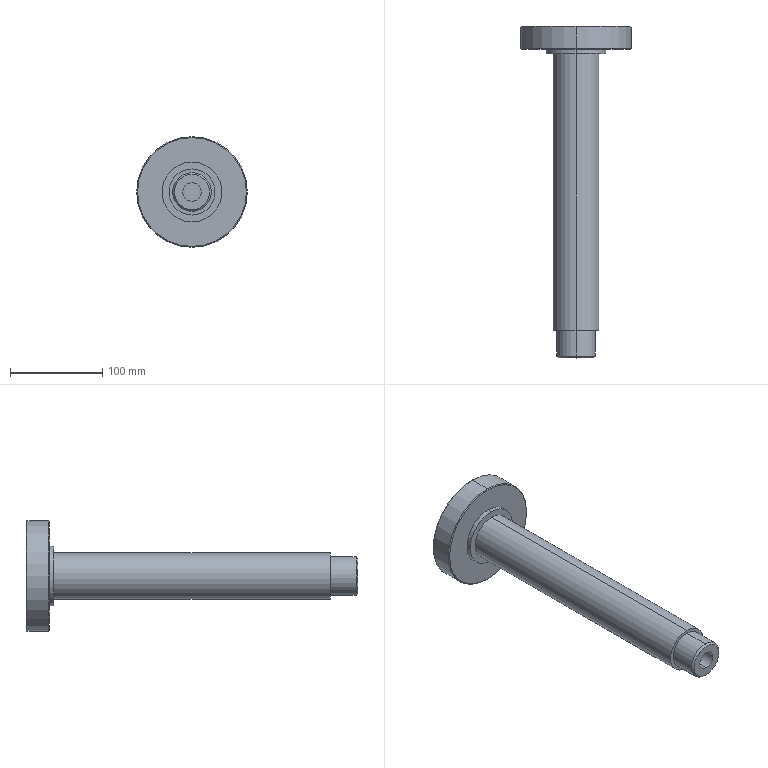Part | STEP file | Backup 2012-3-22-04 | 1 solid | 22 faces | box 120 x 360 x 120 mm | volume 913608 mm3 | cylinder 10 | cone 6 | plane 6 | commonest cylinder face diameters 20 x2 42 x2 50 x2 65 x2 120 x2
STEP:
#1=CARTESIAN_POINT('',(0.,0.,0.));
#2=DIRECTION('',(0.,0.,1.));
#3=DIRECTION('',(1.,0.,0.));
#4=AXIS2_PLACEMENT_3D('',#1,#2,#3);
#5=CARTESIAN_POINT('',(0.,0.,-19.));
#6=VERTEX_POINT('',#5);
#7=CARTESIAN_POINT('',(0.,0.,19.));
#8=VERTEX_POINT('',#7);
#9=CARTESIAN_POINT('',(0.,0.,0.));
#10=DIRECTION('',(0.,-1.,0.));
#11=DIRECTION('',(0.,0.,-1.));
#12=AXIS2_PLACEMENT_3D('',#9,#10,#11);
#13=CIRCLE('',#12,19.);
#14=CARTESIAN_POINT('',(0.,0.,0.));
#15=DIRECTION('',(0.,1.,0.));
#16=DIRECTION('',(0.,0.,1.));
#17=AXIS2_PLACEMENT_3D('',#14,#15,#16);
#18=CONICAL_SURFACE('',#17,19.,0.7854);
#19=CARTESIAN_POINT('',(3.142,0.));
#20=DIRECTION('',(-1.,0.));
#21=VECTOR('',#20,1.);
#22=LINE('',#19,#21);
#23=(GEOMETRIC_REPRESENTATION_CONTEXT(2)PARAMETRIC_REPRESENTATION_CONTEXT()REPRESENTATION_CONTEXT('',''));
#24=DEFINITIONAL_REPRESENTATION('',(#22),#23);
#25=PCURVE('',#18,#24);
#26=CARTESIAN_POINT('',(10.,0.,0.));
#27=DIRECTION('',(0.,-1.,0.));
#28=DIRECTION('',(0.,0.,-1.));
#29=AXIS2_PLACEMENT_3D('',#26,#27,#28);
#30=PLANE('',#29);
#31=CARTESIAN_POINT('',(0.,-10.));
#32=DIRECTION('',(1.,0.));
#33=AXIS2_PLACEMENT_2D('',#31,#32);
#34=CIRCLE('',#33,19.);
#35=(GEOMETRIC_REPRESENTATION_CONTEXT(2)PARAMETRIC_REPRESENTATION_CONTEXT()REPRESENTATION_CONTEXT('',''));
#36=DEFINITIONAL_REPRESENTATION('',(#34),#35);
#37=PCURVE('',#30,#36);
#38=SURFACE_CURVE('',#13,(#25,#37),.PCURVE_S1.);
#39=EDGE_CURVE('',#6,#8,#38,.T.);
#40=ORIENTED_EDGE('',*,*,#39,.F.);
#41=CARTESIAN_POINT('',(0.,2.,-21.));
#42=VERTEX_POINT('',#41);
#43=CARTESIAN_POINT('',(0.,0.,-19.));
#44=DIRECTION('',(0.,0.7071,-0.7071));
#45=VECTOR('',#44,1.);
#46=LINE('',#43,#45);
#47=CARTESIAN_POINT('',(3.142,0.));
#48=DIRECTION('',(0.,1.));
#49=VECTOR('',#48,1.);
#50=LINE('',#47,#49);
#51=(GEOMETRIC_REPRESENTATION_CONTEXT(2)PARAMETRIC_REPRESENTATION_CONTEXT()REPRESENTATION_CONTEXT('',''));
#52=DEFINITIONAL_REPRESENTATION('',(#50),#51);
#53=PCURVE('',#18,#52);
#54=CARTESIAN_POINT('',(0.,0.,0.));
#55=DIRECTION('',(0.,1.,0.));
#56=DIRECTION('',(0.,0.,1.));
#57=AXIS2_PLACEMENT_3D('',#54,#55,#56);
#58=CONICAL_SURFACE('',#57,19.,0.7854);
#59=CARTESIAN_POINT('',(3.142,0.));
#60=DIRECTION('',(0.,1.));
#61=VECTOR('',#60,1.);
#62=LINE('',#59,#61);
#63=(GEOMETRIC_REPRESENTATION_CONTEXT(2)PARAMETRIC_REPRESENTATION_CONTEXT()REPRESENTATION_CONTEXT('',''));
#64=DEFINITIONAL_REPRESENTATION('',(#62),#63);
#65=PCURVE('',#58,#64);
#66=SURFACE_CURVE('',#46,(#53,#65),.PCURVE_S1.);
#67=EDGE_CURVE('',#6,#42,#66,.T.);
#68=ORIENTED_EDGE('',*,*,#67,.T.);
#69=CARTESIAN_POINT('',(0.,2.,21.));
#70=VERTEX_POINT('',#69);
#71=CARTESIAN_POINT('',(0.,2.,0.));
#72=DIRECTION('',(0.,1.,0.));
#73=DIRECTION('',(0.,0.,-1.));
#74=AXIS2_PLACEMENT_3D('',#71,#72,#73);
#75=CIRCLE('',#74,21.);
#76=CARTESIAN_POINT('',(-3.142,2.));
#77=DIRECTION('',(1.,0.));
#78=VECTOR('',#77,1.);
#79=LINE('',#76,#78);
#80=(GEOMETRIC_REPRESENTATION_CONTEXT(2)PARAMETRIC_REPRESENTATION_CONTEXT()REPRESENTATION_CONTEXT('',''));
#81=DEFINITIONAL_REPRESENTATION('',(#79),#80);
#82=PCURVE('',#18,#81);
#83=CARTESIAN_POINT('',(0.,0.,0.));
#84=DIRECTION('',(0.,-1.,0.));
#85=DIRECTION('',(0.,0.,-1.));
#86=AXIS2_PLACEMENT_3D('',#83,#84,#85);
#87=CYLINDRICAL_SURFACE('',#86,21.);
#88=CARTESIAN_POINT('',(6.283,-2.));
#89=DIRECTION('',(-1.,0.));
#90=VECTOR('',#89,1.);
#91=LINE('',#88,#90);
#92=(GEOMETRIC_REPRESENTATION_CONTEXT(2)PARAMETRIC_REPRESENTATION_CONTEXT()REPRESENTATION_CONTEXT('',''));
#93=DEFINITIONAL_REPRESENTATION('',(#91),#92);
#94=PCURVE('',#87,#93);
#95=SURFACE_CURVE('',#75,(#82,#94),.PCURVE_S1.);
#96=EDGE_CURVE('',#70,#42,#95,.T.);
#97=ORIENTED_EDGE('',*,*,#96,.F.);
#98=CARTESIAN_POINT('',(0.,0.,19.));
#99=DIRECTION('',(0.,0.7071,0.7071));
#100=VECTOR('',#99,1.);
#101=LINE('',#98,#100);
#102=CARTESIAN_POINT('',(0.,0.));
#103=DIRECTION('',(0.,1.));
#104=VECTOR('',#103,1.);
#105=LINE('',#102,#104);
#106=(GEOMETRIC_REPRESENTATION_CONTEXT(2)PARAMETRIC_REPRESENTATION_CONTEXT()REPRESENTATION_CONTEXT('',''));
#107=DEFINITIONAL_REPRESENTATION('',(#105),#106);
#108=PCURVE('',#18,#107);
#109=CARTESIAN_POINT('',(6.283,0.));
#110=DIRECTION('',(0.,1.));
#111=VECTOR('',#110,1.);
#112=LINE('',#109,#111);
#113=(GEOMETRIC_REPRESENTATION_CONTEXT(2)PARAMETRIC_REPRESENTATION_CONTEXT()REPRESENTATION_CONTEXT('',''));
#114=DEFINITIONAL_REPRESENTATION('',(#112),#113);
#115=PCURVE('',#58,#114);
#116=SURFACE_CURVE('',#101,(#108,#115),.PCURVE_S1.);
#117=EDGE_CURVE('',#8,#70,#116,.T.);
#118=ORIENTED_EDGE('',*,*,#117,.F.);
#119=EDGE_LOOP('',(#40,#68,#97,#118));
#120=FACE_BOUND('',#119,.T.);
#121=ADVANCED_FACE('',(#120),#18,.T.);
#122=CARTESIAN_POINT('',(0.,360.,59.));
#123=VERTEX_POINT('',#122);
#124=CARTESIAN_POINT('',(0.,360.,-59.));
#125=VERTEX_POINT('',#124);
#126=CARTESIAN_POINT('',(0.,360.,0.));
#127=DIRECTION('',(0.,1.,0.));
#128=DIRECTION('',(0.,0.,1.));
#129=AXIS2_PLACEMENT_3D('',#126,#127,#128);
#130=CIRCLE('',#129,59.);
#131=CARTESIAN_POINT('',(0.,359.,0.));
#132=DIRECTION('',(0.,-1.,0.));
#133=DIRECTION('',(0.,0.,-1.));
#134=AXIS2_PLACEMENT_3D('',#131,#132,#133);
#135=CONICAL_SURFACE('',#134,60.,0.7854);
#136=CARTESIAN_POINT('',(3.142,-1.));
#137=DIRECTION('',(-1.,0.));
#138=VECTOR('',#137,1.);
#139=LINE('',#136,#138);
#140=(GEOMETRIC_REPRESENTATION_CONTEXT(2)PARAMETRIC_REPRESENTATION_CONTEXT()REPRESENTATION_CONTEXT('',''));
#141=DEFINITIONAL_REPRESENTATION('',(#139),#140);
#142=PCURVE('',#135,#141);
#143=CARTESIAN_POINT('',(0.,360.,0.));
#144=DIRECTION('',(0.,1.,0.));
#145=DIRECTION('',(0.,0.,1.));
#146=AXIS2_PLACEMENT_3D('',#143,#144,#145);
#147=PLANE('',#146);
#148=CARTESIAN_POINT('',(0.,0.));
#149=DIRECTION('',(1.,0.));
#150=AXIS2_PLACEMENT_2D('',#148,#149);
#151=CIRCLE('',#150,59.);
#152=(GEOMETRIC_REPRESENTATION_CONTEXT(2)PARAMETRIC_REPRESENTATION_CONTEXT()REPRESENTATION_CONTEXT('',''));
#153=DEFINITIONAL_REPRESENTATION('',(#151),#152);
#154=PCURVE('',#147,#153);
#155=SURFACE_CURVE('',#130,(#142,#154),.PCURVE_S1.);
#156=EDGE_CURVE('',#123,#125,#155,.T.);
#157=ORIENTED_EDGE('',*,*,#156,.F.);
#158=CARTESIAN_POINT('',(0.,359.,60.));
#159=VERTEX_POINT('',#158);
#160=CARTESIAN_POINT('',(0.,359.,60.));
#161=DIRECTION('',(0.,-0.7071,0.7071));
#162=VECTOR('',#161,1.);
#163=LINE('',#160,#162);
#164=CARTESIAN_POINT('',(3.142,0.));
#165=DIRECTION('',(0.,1.));
#166=VECTOR('',#165,1.);
#167=LINE('',#164,#166);
#168=(GEOMETRIC_REPRESENTATION_CONTEXT(2)PARAMETRIC_REPRESENTATION_CONTEXT()REPRESENTATION_CONTEXT('',''));
#169=DEFINITIONAL_REPRESENTATION('',(#167),#168);
#170=PCURVE('',#135,#169);
#171=CARTESIAN_POINT('',(0.,359.,0.));
#172=DIRECTION('',(0.,-1.,0.));
#173=DIRECTION('',(0.,0.,-1.));
#174=AXIS2_PLACEMENT_3D('',#171,#172,#173);
#175=CONICAL_SURFACE('',#174,60.,0.7854);
#176=CARTESIAN_POINT('',(3.142,0.));
#177=DIRECTION('',(0.,1.));
#178=VECTOR('',#177,1.);
#179=LINE('',#176,#178);
#180=(GEOMETRIC_REPRESENTATION_CONTEXT(2)PARAMETRIC_REPRESENTATION_CONTEXT()REPRESENTATION_CONTEXT('',''));
#181=DEFINITIONAL_REPRESENTATION('',(#179),#180);
#182=PCURVE('',#175,#181);
#183=SURFACE_CURVE('',#163,(#170,#182),.PCURVE_S1.);
#184=EDGE_CURVE('',#123,#159,#183,.T.);
#185=ORIENTED_EDGE('',*,*,#184,.T.);
#186=CARTESIAN_POINT('',(0.,359.,-60.));
#187=VERTEX_POINT('',#186);
#188=CARTESIAN_POINT('',(0.,359.,0.));
#189=DIRECTION('',(0.,-1.,0.));
#190=DIRECTION('',(0.,0.,1.));
#191=AXIS2_PLACEMENT_3D('',#188,#189,#190);
#192=CIRCLE('',#191,60.);
#193=CARTESIAN_POINT('',(-3.142,0.));
#194=DIRECTION('',(1.,0.));
#195=VECTOR('',#194,1.);
#196=LINE('',#193,#195);
#197=(GEOMETRIC_REPRESENTATION_CONTEXT(2)PARAMETRIC_REPRESENTATION_CONTEXT()REPRESENTATION_CONTEXT('',''));
#198=DEFINITIONAL_REPRESENTATION('',(#196),#197);
#199=PCURVE('',#135,#198);
#200=CARTESIAN_POINT('',(0.,0.,0.));
#201=DIRECTION('',(0.,-1.,0.));
#202=DIRECTION('',(0.,0.,-1.));
#203=AXIS2_PLACEMENT_3D('',#200,#201,#202);
#204=CYLINDRICAL_SURFACE('',#203,60.);
#205=CARTESIAN_POINT('',(-3.142,-359.));
#206=DIRECTION('',(1.,0.));
#207=VECTOR('',#206,1.);
#208=LINE('',#205,#207);
#209=(GEOMETRIC_REPRESENTATION_CONTEXT(2)PARAMETRIC_REPRESENTATION_CONTEXT()REPRESENTATION_CONTEXT('',''));
#210=DEFINITIONAL_REPRESENTATION('',(#208),#209);
#211=PCURVE('',#204,#210);
#212=SURFACE_CURVE('',#192,(#199,#211),.PCURVE_S1.);
#213=EDGE_CURVE('',#187,#159,#212,.T.);
#214=ORIENTED_EDGE('',*,*,#213,.F.);
#215=CARTESIAN_POINT('',(0.,359.,-60.));
#216=DIRECTION('',(0.,-0.7071,-0.7071));
#217=VECTOR('',#216,1.);
#218=LINE('',#215,#217);
#219=CARTESIAN_POINT('',(0.,0.));
#220=DIRECTION('',(0.,1.));
#221=VECTOR('',#220,1.);
#222=LINE('',#219,#221);
#223=(GEOMETRIC_REPRESENTATION_CONTEXT(2)PARAMETRIC_REPRESENTATION_CONTEXT()REPRESENTATION_CONTEXT('',''));
#224=DEFINITIONAL_REPRESENTATION('',(#222),#223);
#225=PCURVE('',#135,#224);
#226=CARTESIAN_POINT('',(6.283,0.));
#227=DIRECTION('',(0.,1.));
#228=VECTOR('',#227,1.);
#229=LINE('',#226,#228);
#230=(GEOMETRIC_REPRESENTATION_CONTEXT(2)PARAMETRIC_REPRESENTATION_CONTEXT()REPRESENTATION_CONTEXT('',''));
#231=DEFINITIONAL_REPRESENTATION('',(#229),#230);
#232=PCURVE('',#175,#231);
#233=SURFACE_CURVE('',#218,(#225,#232),.PCURVE_S1.);
#234=EDGE_CURVE('',#125,#187,#233,.T.);
#235=ORIENTED_EDGE('',*,*,#234,.F.);
#236=EDGE_LOOP('',(#157,#185,#214,#235));
#237=FACE_BOUND('',#236,.T.);
#238=ADVANCED_FACE('',(#237),#135,.T.);
#239=CARTESIAN_POINT('',(0.,335.,-59.));
#240=VERTEX_POINT('',#239);
#241=CARTESIAN_POINT('',(0.,335.,59.));
#242=VERTEX_POINT('',#241);
#243=CARTESIAN_POINT('',(0.,335.,0.));
#244=DIRECTION('',(0.,-1.,0.));
#245=DIRECTION('',(0.,0.,-1.));
#246=AXIS2_PLACEMENT_3D('',#243,#244,#245);
#247=CIRCLE('',#246,59.);
#248=CARTESIAN_POINT('',(0.,335.,0.));
#249=DIRECTION('',(0.,1.,0.));
#250=DIRECTION('',(0.,0.,1.));
#251=AXIS2_PLACEMENT_3D('',#248,#249,#250);
#252=CONICAL_SURFACE('',#251,59.,0.7854);
#253=CARTESIAN_POINT('',(3.142,0.));
#254=DIRECTION('',(-1.,0.));
#255=VECTOR('',#254,1.);
#256=LINE('',#253,#255);
#257=(GEOMETRIC_REPRESENTATION_CONTEXT(2)PARAMETRIC_REPRESENTATION_CONTEXT()REPRESENTATION_CONTEXT('',''));
#258=DEFINITIONAL_REPRESENTATION('',(#256),#257);
#259=PCURVE('',#252,#258);
#260=CARTESIAN_POINT('',(32.5,335.,0.));
#261=DIRECTION('',(0.,-1.,0.));
#262=DIRECTION('',(0.,0.,-1.));
#263=AXIS2_PLACEMENT_3D('',#260,#261,#262);
#264=PLANE('',#263);
#265=CARTESIAN_POINT('',(0.,-32.5));
#266=DIRECTION('',(1.,0.));
#267=AXIS2_PLACEMENT_2D('',#265,#266);
#268=CIRCLE('',#267,59.);
#269=(GEOMETRIC_REPRESENTATION_CONTEXT(2)PARAMETRIC_REPRESENTATION_CONTEXT()REPRESENTATION_CONTEXT('',''));
#270=DEFINITIONAL_REPRESENTATION('',(#268),#269);
#271=PCURVE('',#264,#270);
#272=SURFACE_CURVE('',#247,(#259,#271),.PCURVE_S1.);
#273=EDGE_CURVE('',#240,#242,#272,.T.);
#274=ORIENTED_EDGE('',*,*,#273,.F.);
#275=CARTESIAN_POINT('',(0.,336.,-60.));
#276=VERTEX_POINT('',#275);
#277=CARTESIAN_POINT('',(0.,335.,-59.));
#278=DIRECTION('',(0.,0.7071,-0.7071));
#279=VECTOR('',#278,1.);
#280=LINE('',#277,#279);
#281=CARTESIAN_POINT('',(3.142,0.));
#282=DIRECTION('',(0.,1.));
#283=VECTOR('',#282,1.);
#284=LINE('',#281,#283);
#285=(GEOMETRIC_REPRESENTATION_CONTEXT(2)PARAMETRIC_REPRESENTATION_CONTEXT()REPRESENTATION_CONTEXT('',''));
#286=DEFINITIONAL_REPRESENTATION('',(#284),#285);
#287=PCURVE('',#252,#286);
#288=CARTESIAN_POINT('',(0.,335.,0.));
#289=DIRECTION('',(0.,1.,0.));
#290=DIRECTION('',(0.,0.,1.));
#291=AXIS2_PLACEMENT_3D('',#288,#289,#290);
#292=CONICAL_SURFACE('',#291,59.,0.7854);
#293=CARTESIAN_POINT('',(3.142,0.));
#294=DIRECTION('',(0.,1.));
#295=VECTOR('',#294,1.);
#296=LINE('',#293,#295);
#297=(GEOMETRIC_REPRESENTATION_CONTEXT(2)PARAMETRIC_REPRESENTATION_CONTEXT()REPRESENTATION_CONTEXT('',''));
#298=DEFINITIONAL_REPRESENTATION('',(#296),#297);
#299=PCURVE('',#292,#298);
#300=SURFACE_CURVE('',#280,(#287,#299),.PCURVE_S1.);
#301=EDGE_CURVE('',#240,#276,#300,.T.);
#302=ORIENTED_EDGE('',*,*,#301,.T.);
#303=CARTESIAN_POINT('',(0.,336.,60.));
#304=VERTEX_POINT('',#303);
#305=CARTESIAN_POINT('',(0.,336.,0.));
#306=DIRECTION('',(0.,1.,0.));
#307=DIRECTION('',(0.,0.,-1.));
#308=AXIS2_PLACEMENT_3D('',#305,#306,#307);
#309=CIRCLE('',#308,60.);
#310=CARTESIAN_POINT('',(-3.142,1.));
#311=DIRECTION('',(1.,0.));
#312=VECTOR('',#311,1.);
#313=LINE('',#310,#312);
#314=(GEOMETRIC_REPRESENTATION_CONTEXT(2)PARAMETRIC_REPRESENTATION_CONTEXT()REPRESENTATION_CONTEXT('',''));
#315=DEFINITIONAL_REPRESENTATION('',(#313),#314);
#316=PCURVE('',#252,#315);
#317=CARTESIAN_POINT('',(6.283,-336.));
#318=DIRECTION('',(-1.,0.));
#319=VECTOR('',#318,1.);
#320=LINE('',#317,#319);
#321=(GEOMETRIC_REPRESENTATION_CONTEXT(2)PARAMETRIC_REPRESENTATION_CONTEXT()REPRESENTATION_CONTEXT('',''));
#322=DEFINITIONAL_REPRESENTATION('',(#320),#321);
#323=PCURVE('',#204,#322);
#324=SURFACE_CURVE('',#309,(#316,#323),.PCURVE_S1.);
#325=EDGE_CURVE('',#304,#276,#324,.T.);
#326=ORIENTED_EDGE('',*,*,#325,.F.);
#327=CARTESIAN_POINT('',(0.,335.,59.));
#328=DIRECTION('',(0.,0.7071,0.7071));
#329=VECTOR('',#328,1.);
#330=LINE('',#327,#329);
#331=CARTESIAN_POINT('',(0.,0.));
#332=DIRECTION('',(0.,1.));
#333=VECTOR('',#332,1.);
#334=LINE('',#331,#333);
#335=(GEOMETRIC_REPRESENTATION_CONTEXT(2)PARAMETRIC_REPRESENTATION_CONTEXT()REPRESENTATION_CONTEXT('',''));
#336=DEFINITIONAL_REPRESENTATION('',(#334),#335);
#337=PCURVE('',#252,#336);
#338=CARTESIAN_POINT('',(6.283,0.));
#339=DIRECTION('',(0.,1.));
#340=VECTOR('',#339,1.);
#341=LINE('',#338,#340);
#342=(GEOMETRIC_REPRESENTATION_CONTEXT(2)PARAMETRIC_REPRESENTATION_CONTEXT()REPRESENTATION_CONTEXT('',''));
#343=DEFINITIONAL_REPRESENTATION('',(#341),#342);
#344=PCURVE('',#292,#343);
#345=SURFACE_CURVE('',#330,(#337,#344),.PCURVE_S1.);
#346=EDGE_CURVE('',#242,#304,#345,.T.);
#347=ORIENTED_EDGE('',*,*,#346,.F.);
#348=EDGE_LOOP('',(#274,#302,#326,#347));
#349=FACE_BOUND('',#348,.T.);
#350=ADVANCED_FACE('',(#349),#252,.T.);
#351=ORIENTED_EDGE('',*,*,#213,.T.);
#352=CARTESIAN_POINT('',(0.,0.,60.));
#353=DIRECTION('',(0.,-1.,0.));
#354=VECTOR('',#353,1.);
#355=LINE('',#352,#354);
#356=CARTESIAN_POINT('',(3.142,0.));
#357=DIRECTION('',(0.,1.));
#358=VECTOR('',#357,1.);
#359=LINE('',#356,#358);
#360=(GEOMETRIC_REPRESENTATION_CONTEXT(2)PARAMETRIC_REPRESENTATION_CONTEXT()REPRESENTATION_CONTEXT('',''));
#361=DEFINITIONAL_REPRESENTATION('',(#359),#360);
#362=PCURVE('',#204,#361);
#363=CARTESIAN_POINT('',(0.,0.,0.));
#364=DIRECTION('',(0.,-1.,0.));
#365=DIRECTION('',(0.,0.,-1.));
#366=AXIS2_PLACEMENT_3D('',#363,#364,#365);
#367=CYLINDRICAL_SURFACE('',#366,60.);
#368=CARTESIAN_POINT('',(3.142,0.));
#369=DIRECTION('',(0.,1.));
#370=VECTOR('',#369,1.);
#371=LINE('',#368,#370);
#372=(GEOMETRIC_REPRESENTATION_CONTEXT(2)PARAMETRIC_REPRESENTATION_CONTEXT()REPRESENTATION_CONTEXT('',''));
#373=DEFINITIONAL_REPRESENTATION('',(#371),#372);
#374=PCURVE('',#367,#373);
#375=SURFACE_CURVE('',#355,(#362,#374),.PCURVE_S1.);
#376=EDGE_CURVE('',#159,#304,#375,.T.);
#377=ORIENTED_EDGE('',*,*,#376,.T.);
#378=ORIENTED_EDGE('',*,*,#325,.T.);
#379=CARTESIAN_POINT('',(0.,0.,-60.));
#380=DIRECTION('',(0.,-1.,0.));
#381=VECTOR('',#380,1.);
#382=LINE('',#379,#381);
#383=CARTESIAN_POINT('',(0.,0.));
#384=DIRECTION('',(0.,1.));
#385=VECTOR('',#384,1.);
#386=LINE('',#383,#385);
#387=(GEOMETRIC_REPRESENTATION_CONTEXT(2)PARAMETRIC_REPRESENTATION_CONTEXT()REPRESENTATION_CONTEXT('',''));
#388=DEFINITIONAL_REPRESENTATION('',(#386),#387);
#389=PCURVE('',#204,#388);
#390=CARTESIAN_POINT('',(6.283,0.));
#391=DIRECTION('',(0.,1.));
#392=VECTOR('',#391,1.);
#393=LINE('',#390,#392);
#394=(GEOMETRIC_REPRESENTATION_CONTEXT(2)PARAMETRIC_REPRESENTATION_CONTEXT()REPRESENTATION_CONTEXT('',''));
#395=DEFINITIONAL_REPRESENTATION('',(#393),#394);
#396=PCURVE('',#367,#395);
#397=SURFACE_CURVE('',#382,(#389,#396),.PCURVE_S1.);
#398=EDGE_CURVE('',#187,#276,#397,.T.);
#399=ORIENTED_EDGE('',*,*,#398,.F.);
#400=EDGE_LOOP('',(#351,#377,#378,#399));
#401=FACE_BOUND('',#400,.T.);
#402=ADVANCED_FACE('',(#401),#204,.T.);
#403=CARTESIAN_POINT('',(0.,335.,-32.5));
#404=VERTEX_POINT('',#403);
#405=CARTESIAN_POINT('',(0.,335.,32.5));
#406=VERTEX_POINT('',#405);
#407=CARTESIAN_POINT('',(0.,335.,0.));
#408=DIRECTION('',(0.,-1.,0.));
#409=DIRECTION('',(0.,0.,-1.));
#410=AXIS2_PLACEMENT_3D('',#407,#408,#409);
#411=CIRCLE('',#410,32.5);
#412=CARTESIAN_POINT('',(0.,0.,0.));
#413=DIRECTION('',(0.,-1.,0.));
#414=DIRECTION('',(0.,0.,-1.));
#415=AXIS2_PLACEMENT_3D('',#412,#413,#414);
#416=CYLINDRICAL_SURFACE('',#415,32.5);
#417=CARTESIAN_POINT('',(0.,-335.));
#418=DIRECTION('',(1.,0.));
#419=VECTOR('',#418,1.);
#420=LINE('',#417,#419);
#421=(GEOMETRIC_REPRESENTATION_CONTEXT(2)PARAMETRIC_REPRESENTATION_CONTEXT()REPRESENTATION_CONTEXT('',''));
#422=DEFINITIONAL_REPRESENTATION('',(#420),#421);
#423=PCURVE('',#416,#422);
#424=CARTESIAN_POINT('',(0.,-32.5));
#425=DIRECTION('',(1.,0.));
#426=AXIS2_PLACEMENT_2D('',#424,#425);
#427=CIRCLE('',#426,32.5);
#428=(GEOMETRIC_REPRESENTATION_CONTEXT(2)PARAMETRIC_REPRESENTATION_CONTEXT()REPRESENTATION_CONTEXT('',''));
#429=DEFINITIONAL_REPRESENTATION('',(#427),#428);
#430=PCURVE('',#264,#429);
#431=SURFACE_CURVE('',#411,(#423,#430),.PCURVE_S1.);
#432=EDGE_CURVE('',#404,#406,#431,.T.);
#433=ORIENTED_EDGE('',*,*,#432,.T.);
#434=CARTESIAN_POINT('',(0.,330.,32.5));
#435=VERTEX_POINT('',#434);
#436=CARTESIAN_POINT('',(0.,0.,32.5));
#437=DIRECTION('',(0.,-1.,0.));
#438=VECTOR('',#437,1.);
#439=LINE('',#436,#438);
#440=CARTESIAN_POINT('',(3.142,0.));
#441=DIRECTION('',(0.,1.));
#442=VECTOR('',#441,1.);
#443=LINE('',#440,#442);
#444=(GEOMETRIC_REPRESENTATION_CONTEXT(2)PARAMETRIC_REPRESENTATION_CONTEXT()REPRESENTATION_CONTEXT('',''));
#445=DEFINITIONAL_REPRESENTATION('',(#443),#444);
#446=PCURVE('',#416,#445);
#447=CARTESIAN_POINT('',(0.,0.,0.));
#448=DIRECTION('',(0.,-1.,0.));
#449=DIRECTION('',(0.,0.,-1.));
#450=AXIS2_PLACEMENT_3D('',#447,#448,#449);
#451=CYLINDRICAL_SURFACE('',#450,32.5);
#452=CARTESIAN_POINT('',(3.142,0.));
#453=DIRECTION('',(0.,1.));
#454=VECTOR('',#453,1.);
#455=LINE('',#452,#454);
#456=(GEOMETRIC_REPRESENTATION_CONTEXT(2)PARAMETRIC_REPRESENTATION_CONTEXT()REPRESENTATION_CONTEXT('',''));
#457=DEFINITIONAL_REPRESENTATION('',(#455),#456);
#458=PCURVE('',#451,#457);
#459=SURFACE_CURVE('',#439,(#446,#458),.PCURVE_S1.);
#460=EDGE_CURVE('',#406,#435,#459,.T.);
#461=ORIENTED_EDGE('',*,*,#460,.T.);
#462=CARTESIAN_POINT('',(0.,330.,-32.5));
#463=VERTEX_POINT('',#462);
#464=CARTESIAN_POINT('',(0.,330.,0.));
#465=DIRECTION('',(0.,-1.,0.));
#466=DIRECTION('',(0.,0.,-1.));
#467=AXIS2_PLACEMENT_3D('',#464,#465,#466);
#468=CIRCLE('',#467,32.5);
#469=CARTESIAN_POINT('',(0.,-330.));
#470=DIRECTION('',(1.,0.));
#471=VECTOR('',#470,1.);
#472=LINE('',#469,#471);
#473=(GEOMETRIC_REPRESENTATION_CONTEXT(2)PARAMETRIC_REPRESENTATION_CONTEXT()REPRESENTATION_CONTEXT('',''));
#474=DEFINITIONAL_REPRESENTATION('',(#472),#473);
#475=PCURVE('',#416,#474);
#476=CARTESIAN_POINT('',(25.,330.,0.));
#477=DIRECTION('',(0.,-1.,0.));
#478=DIRECTION('',(0.,0.,-1.));
#479=AXIS2_PLACEMENT_3D('',#476,#477,#478);
#480=PLANE('',#479);
#481=CARTESIAN_POINT('',(0.,-25.));
#482=DIRECTION('',(1.,0.));
#483=AXIS2_PLACEMENT_2D('',#481,#482);
#484=CIRCLE('',#483,32.5);
#485=(GEOMETRIC_REPRESENTATION_CONTEXT(2)PARAMETRIC_REPRESENTATION_CONTEXT()REPRESENTATION_CONTEXT('',''));
#486=DEFINITIONAL_REPRESENTATION('',(#484),#485);
#487=PCURVE('',#480,#486);
#488=SURFACE_CURVE('',#468,(#475,#487),.PCURVE_S1.);
#489=EDGE_CURVE('',#463,#435,#488,.T.);
#490=ORIENTED_EDGE('',*,*,#489,.F.);
#491=CARTESIAN_POINT('',(0.,0.,-32.5));
#492=DIRECTION('',(0.,-1.,0.));
#493=VECTOR('',#492,1.);
#494=LINE('',#491,#493);
#495=CARTESIAN_POINT('',(0.,0.));
#496=DIRECTION('',(0.,1.));
#497=VECTOR('',#496,1.);
#498=LINE('',#495,#497);
#499=(GEOMETRIC_REPRESENTATION_CONTEXT(2)PARAMETRIC_REPRESENTATION_CONTEXT()REPRESENTATION_CONTEXT('',''));
#500=DEFINITIONAL_REPRESENTATION('',(#498),#499);
#501=PCURVE('',#416,#500);
#502=CARTESIAN_POINT('',(6.283,0.));
#503=DIRECTION('',(0.,1.));
#504=VECTOR('',#503,1.);
#505=LINE('',#502,#504);
#506=(GEOMETRIC_REPRESENTATION_CONTEXT(2)PARAMETRIC_REPRESENTATION_CONTEXT()REPRESENTATION_CONTEXT('',''));
#507=DEFINITIONAL_REPRESENTATION('',(#505),#506);
#508=PCURVE('',#451,#507);
#509=SURFACE_CURVE('',#494,(#501,#508),.PCURVE_S1.);
#510=EDGE_CURVE('',#404,#463,#509,.T.);
#511=ORIENTED_EDGE('',*,*,#510,.F.);
#512=EDGE_LOOP('',(#433,#461,#490,#511));
#513=FACE_BOUND('',#512,.T.);
#514=ADVANCED_FACE('',(#513),#416,.T.);
#515=CARTESIAN_POINT('',(0.,330.,-25.));
#516=VERTEX_POINT('',#515);
#517=CARTESIAN_POINT('',(0.,330.,25.));
#518=VERTEX_POINT('',#517);
#519=CARTESIAN_POINT('',(0.,330.,0.));
#520=DIRECTION('',(0.,-1.,0.));
#521=DIRECTION('',(0.,0.,-1.));
#522=AXIS2_PLACEMENT_3D('',#519,#520,#521);
#523=CIRCLE('',#522,25.);
#524=CARTESIAN_POINT('',(0.,0.,0.));
#525=DIRECTION('',(0.,-1.,0.));
#526=DIRECTION('',(0.,0.,-1.));
#527=AXIS2_PLACEMENT_3D('',#524,#525,#526);
#528=CYLINDRICAL_SURFACE('',#527,25.);
#529=CARTESIAN_POINT('',(0.,-330.));
#530=DIRECTION('',(1.,0.));
#531=VECTOR('',#530,1.);
#532=LINE('',#529,#531);
#533=(GEOMETRIC_REPRESENTATION_CONTEXT(2)PARAMETRIC_REPRESENTATION_CONTEXT()REPRESENTATION_CONTEXT('',''));
#534=DEFINITIONAL_REPRESENTATION('',(#532),#533);
#535=PCURVE('',#528,#534);
#536=CARTESIAN_POINT('',(0.,-25.));
#537=DIRECTION('',(1.,0.));
#538=AXIS2_PLACEMENT_2D('',#536,#537);
#539=CIRCLE('',#538,25.);
#540=(GEOMETRIC_REPRESENTATION_CONTEXT(2)PARAMETRIC_REPRESENTATION_CONTEXT()REPRESENTATION_CONTEXT('',''));
#541=DEFINITIONAL_REPRESENTATION('',(#539),#540);
#542=PCURVE('',#480,#541);
#543=SURFACE_CURVE('',#523,(#535,#542),.PCURVE_S1.);
#544=EDGE_CURVE('',#516,#518,#543,.T.);
#545=ORIENTED_EDGE('',*,*,#544,.T.);
#546=CARTESIAN_POINT('',(0.,30.,25.));
#547=VERTEX_POINT('',#546);
#548=CARTESIAN_POINT('',(0.,0.,25.));
#549=DIRECTION('',(0.,-1.,0.));
#550=VECTOR('',#549,1.);
#551=LINE('',#548,#550);
#552=CARTESIAN_POINT('',(3.142,0.));
#553=DIRECTION('',(0.,1.));
#554=VECTOR('',#553,1.);
#555=LINE('',#552,#554);
#556=(GEOMETRIC_REPRESENTATION_CONTEXT(2)PARAMETRIC_REPRESENTATION_CONTEXT()REPRESENTATION_CONTEXT('',''));
#557=DEFINITIONAL_REPRESENTATION('',(#555),#556);
#558=PCURVE('',#528,#557);
#559=CARTESIAN_POINT('',(0.,0.,0.));
#560=DIRECTION('',(0.,-1.,0.));
#561=DIRECTION('',(0.,0.,-1.));
#562=AXIS2_PLACEMENT_3D('',#559,#560,#561);
#563=CYLINDRICAL_SURFACE('',#562,25.);
#564=CARTESIAN_POINT('',(3.142,0.));
#565=DIRECTION('',(0.,1.));
#566=VECTOR('',#565,1.);
#567=LINE('',#564,#566);
#568=(GEOMETRIC_REPRESENTATION_CONTEXT(2)PARAMETRIC_REPRESENTATION_CONTEXT()REPRESENTATION_CONTEXT('',''));
#569=DEFINITIONAL_REPRESENTATION('',(#567),#568);
#570=PCURVE('',#563,#569);
#571=SURFACE_CURVE('',#551,(#558,#570),.PCURVE_S1.);
#572=EDGE_CURVE('',#518,#547,#571,.T.);
#573=ORIENTED_EDGE('',*,*,#572,.T.);
#574=CARTESIAN_POINT('',(0.,30.,-25.));
#575=VERTEX_POINT('',#574);
#576=CARTESIAN_POINT('',(0.,30.,0.));
#577=DIRECTION('',(0.,-1.,0.));
#578=DIRECTION('',(0.,0.,-1.));
#579=AXIS2_PLACEMENT_3D('',#576,#577,#578);
#580=CIRCLE('',#579,25.);
#581=CARTESIAN_POINT('',(0.,-30.));
#582=DIRECTION('',(1.,0.));
#583=VECTOR('',#582,1.);
#584=LINE('',#581,#583);
#585=(GEOMETRIC_REPRESENTATION_CONTEXT(2)PARAMETRIC_REPRESENTATION_CONTEXT()REPRESENTATION_CONTEXT('',''));
#586=DEFINITIONAL_REPRESENTATION('',(#584),#585);
#587=PCURVE('',#528,#586);
#588=CARTESIAN_POINT('',(21.,30.,0.));
#589=DIRECTION('',(0.,-1.,0.));
#590=DIRECTION('',(0.,0.,-1.));
#591=AXIS2_PLACEMENT_3D('',#588,#589,#590);
#592=PLANE('',#591);
#593=CARTESIAN_POINT('',(0.,-21.));
#594=DIRECTION('',(1.,0.));
#595=AXIS2_PLACEMENT_2D('',#593,#594);
#596=CIRCLE('',#595,25.);
#597=(GEOMETRIC_REPRESENTATION_CONTEXT(2)PARAMETRIC_REPRESENTATION_CONTEXT()REPRESENTATION_CONTEXT('',''));
#598=DEFINITIONAL_REPRESENTATION('',(#596),#597);
#599=PCURVE('',#592,#598);
#600=SURFACE_CURVE('',#580,(#587,#599),.PCURVE_S1.);
#601=EDGE_CURVE('',#575,#547,#600,.T.);
#602=ORIENTED_EDGE('',*,*,#601,.F.);
#603=CARTESIAN_POINT('',(0.,0.,-25.));
#604=DIRECTION('',(0.,-1.,0.));
#605=VECTOR('',#604,1.);
#606=LINE('',#603,#605);
#607=CARTESIAN_POINT('',(0.,0.));
#608=DIRECTION('',(0.,1.));
#609=VECTOR('',#608,1.);
#610=LINE('',#607,#609);
#611=(GEOMETRIC_REPRESENTATION_CONTEXT(2)PARAMETRIC_REPRESENTATION_CONTEXT()REPRESENTATION_CONTEXT('',''));
#612=DEFINITIONAL_REPRESENTATION('',(#610),#611);
#613=PCURVE('',#528,#612);
#614=CARTESIAN_POINT('',(6.283,0.));
#615=DIRECTION('',(0.,1.));
#616=VECTOR('',#615,1.);
#617=LINE('',#614,#616);
#618=(GEOMETRIC_REPRESENTATION_CONTEXT(2)PARAMETRIC_REPRESENTATION_CONTEXT()REPRESENTATION_CONTEXT('',''));
#619=DEFINITIONAL_REPRESENTATION('',(#617),#618);
#620=PCURVE('',#563,#619);
#621=SURFACE_CURVE('',#606,(#613,#620),.PCURVE_S1.);
#622=EDGE_CURVE('',#516,#575,#621,.T.);
#623=ORIENTED_EDGE('',*,*,#622,.F.);
#624=EDGE_LOOP('',(#545,#573,#602,#623));
#625=FACE_BOUND('',#624,.T.);
#626=ADVANCED_FACE('',(#625),#528,.T.);
#627=CARTESIAN_POINT('',(0.,30.,-21.));
#628=VERTEX_POINT('',#627);
#629=CARTESIAN_POINT('',(0.,30.,21.));
#630=VERTEX_POINT('',#629);
#631=CARTESIAN_POINT('',(0.,30.,0.));
#632=DIRECTION('',(0.,-1.,0.));
#633=DIRECTION('',(0.,0.,-1.));
#634=AXIS2_PLACEMENT_3D('',#631,#632,#633);
#635=CIRCLE('',#634,21.);
#636=CARTESIAN_POINT('',(0.,-30.));
#637=DIRECTION('',(1.,0.));
#638=VECTOR('',#637,1.);
#639=LINE('',#636,#638);
#640=(GEOMETRIC_REPRESENTATION_CONTEXT(2)PARAMETRIC_REPRESENTATION_CONTEXT()REPRESENTATION_CONTEXT('',''));
#641=DEFINITIONAL_REPRESENTATION('',(#639),#640);
#642=PCURVE('',#87,#641);
#643=CARTESIAN_POINT('',(0.,-21.));
#644=DIRECTION('',(1.,0.));
#645=AXIS2_PLACEMENT_2D('',#643,#644);
#646=CIRCLE('',#645,21.);
#647=(GEOMETRIC_REPRESENTATION_CONTEXT(2)PARAMETRIC_REPRESENTATION_CONTEXT()REPRESENTATION_CONTEXT('',''));
#648=DEFINITIONAL_REPRESENTATION('',(#646),#647);
#649=PCURVE('',#592,#648);
#650=SURFACE_CURVE('',#635,(#642,#649),.PCURVE_S1.);
#651=EDGE_CURVE('',#628,#630,#650,.T.);
#652=ORIENTED_EDGE('',*,*,#651,.T.);
#653=CARTESIAN_POINT('',(0.,0.,21.));
#654=DIRECTION('',(0.,-1.,0.));
#655=VECTOR('',#654,1.);
#656=LINE('',#653,#655);
#657=CARTESIAN_POINT('',(3.142,0.));
#658=DIRECTION('',(0.,1.));
#659=VECTOR('',#658,1.);
#660=LINE('',#657,#659);
#661=(GEOMETRIC_REPRESENTATION_CONTEXT(2)PARAMETRIC_REPRESENTATION_CONTEXT()REPRESENTATION_CONTEXT('',''));
#662=DEFINITIONAL_REPRESENTATION('',(#660),#661);
#663=PCURVE('',#87,#662);
#664=CARTESIAN_POINT('',(0.,0.,0.));
#665=DIRECTION('',(0.,-1.,0.));
#666=DIRECTION('',(0.,0.,-1.));
#667=AXIS2_PLACEMENT_3D('',#664,#665,#666);
#668=CYLINDRICAL_SURFACE('',#667,21.);
#669=CARTESIAN_POINT('',(3.142,0.));
#670=DIRECTION('',(0.,1.));
#671=VECTOR('',#670,1.);
#672=LINE('',#669,#671);
#673=(GEOMETRIC_REPRESENTATION_CONTEXT(2)PARAMETRIC_REPRESENTATION_CONTEXT()REPRESENTATION_CONTEXT('',''));
#674=DEFINITIONAL_REPRESENTATION('',(#672),#673);
#675=PCURVE('',#668,#674);
#676=SURFACE_CURVE('',#656,(#663,#675),.PCURVE_S1.);
#677=EDGE_CURVE('',#630,#70,#676,.T.);
#678=ORIENTED_EDGE('',*,*,#677,.T.);
#679=ORIENTED_EDGE('',*,*,#96,.T.);
#680=CARTESIAN_POINT('',(0.,0.,-21.));
#681=DIRECTION('',(0.,-1.,0.));
#682=VECTOR('',#681,1.);
#683=LINE('',#680,#682);
#684=CARTESIAN_POINT('',(0.,0.));
#685=DIRECTION('',(0.,1.));
#686=VECTOR('',#685,1.);
#687=LINE('',#684,#686);
#688=(GEOMETRIC_REPRESENTATION_CONTEXT(2)PARAMETRIC_REPRESENTATION_CONTEXT()REPRESENTATION_CONTEXT('',''));
#689=DEFINITIONAL_REPRESENTATION('',(#687),#688);
#690=PCURVE('',#87,#689);
#691=CARTESIAN_POINT('',(6.283,0.));
#692=DIRECTION('',(0.,1.));
#693=VECTOR('',#692,1.);
#694=LINE('',#691,#693);
#695=(GEOMETRIC_REPRESENTATION_CONTEXT(2)PARAMETRIC_REPRESENTATION_CONTEXT()REPRESENTATION_CONTEXT('',''));
#696=DEFINITIONAL_REPRESENTATION('',(#694),#695);
#697=PCURVE('',#668,#696);
#698=SURFACE_CURVE('',#683,(#690,#697),.PCURVE_S1.);
#699=EDGE_CURVE('',#628,#42,#698,.T.);
#700=ORIENTED_EDGE('',*,*,#699,.F.);
#701=EDGE_LOOP('',(#652,#678,#679,#700));
#702=FACE_BOUND('',#701,.T.);
#703=ADVANCED_FACE('',(#702),#87,.T.);
#704=CARTESIAN_POINT('',(0.,50.,-10.));
#705=VERTEX_POINT('',#704);
#706=CARTESIAN_POINT('',(0.,0.,-10.));
#707=VERTEX_POINT('',#706);
#708=CARTESIAN_POINT('',(0.,0.,-10.));
#709=DIRECTION('',(0.,-1.,0.));
#710=VECTOR('',#709,1.);
#711=LINE('',#708,#710);
#712=CARTESIAN_POINT('',(0.,0.,0.));
#713=DIRECTION('',(0.,-1.,0.));
#714=DIRECTION('',(0.,0.,-1.));
#715=AXIS2_PLACEMENT_3D('',#712,#713,#714);
#716=CYLINDRICAL_SURFACE('',#715,10.);
#717=CARTESIAN_POINT('',(6.283,0.));
#718=DIRECTION('',(0.,1.));
#719=VECTOR('',#718,1.);
#720=LINE('',#717,#719);
#721=(GEOMETRIC_REPRESENTATION_CONTEXT(2)PARAMETRIC_REPRESENTATION_CONTEXT()REPRESENTATION_CONTEXT('',''));
#722=DEFINITIONAL_REPRESENTATION('',(#720),#721);
#723=PCURVE('',#716,#722);
#724=CARTESIAN_POINT('',(0.,0.,0.));
#725=DIRECTION('',(0.,-1.,0.));
#726=DIRECTION('',(0.,0.,-1.));
#727=AXIS2_PLACEMENT_3D('',#724,#725,#726);
#728=CYLINDRICAL_SURFACE('',#727,10.);
#729=CARTESIAN_POINT('',(0.,0.));
#730=DIRECTION('',(0.,1.));
#731=VECTOR('',#730,1.);
#732=LINE('',#729,#731);
#733=(GEOMETRIC_REPRESENTATION_CONTEXT(2)PARAMETRIC_REPRESENTATION_CONTEXT()REPRESENTATION_CONTEXT('',''));
#734=DEFINITIONAL_REPRESENTATION('',(#732),#733);
#735=PCURVE('',#728,#734);
#736=SURFACE_CURVE('',#711,(#723,#735),.PCURVE_S1.);
#737=EDGE_CURVE('',#705,#707,#736,.T.);
#738=ORIENTED_EDGE('',*,*,#737,.T.);
#739=CARTESIAN_POINT('',(0.,0.,10.));
#740=VERTEX_POINT('',#739);
#741=CARTESIAN_POINT('',(0.,0.,0.));
#742=DIRECTION('',(0.,-1.,0.));
#743=DIRECTION('',(0.,0.,-1.));
#744=AXIS2_PLACEMENT_3D('',#741,#742,#743);
#745=CIRCLE('',#744,10.);
#746=CARTESIAN_POINT('',(0.,0.));
#747=DIRECTION('',(1.,0.));
#748=VECTOR('',#747,1.);
#749=LINE('',#746,#748);
#750=(GEOMETRIC_REPRESENTATION_CONTEXT(2)PARAMETRIC_REPRESENTATION_CONTEXT()REPRESENTATION_CONTEXT('',''));
#751=DEFINITIONAL_REPRESENTATION('',(#749),#750);
#752=PCURVE('',#716,#751);
#753=CARTESIAN_POINT('',(0.,-10.));
#754=DIRECTION('',(1.,0.));
#755=AXIS2_PLACEMENT_2D('',#753,#754);
#756=CIRCLE('',#755,10.);
#757=(GEOMETRIC_REPRESENTATION_CONTEXT(2)PARAMETRIC_REPRESENTATION_CONTEXT()REPRESENTATION_CONTEXT('',''));
#758=DEFINITIONAL_REPRESENTATION('',(#756),#757);
#759=PCURVE('',#30,#758);
#760=SURFACE_CURVE('',#745,(#752,#759),.PCURVE_S1.);
#761=EDGE_CURVE('',#740,#707,#760,.T.);
#762=ORIENTED_EDGE('',*,*,#761,.F.);
#763=CARTESIAN_POINT('',(0.,50.,10.));
#764=VERTEX_POINT('',#763);
#765=CARTESIAN_POINT('',(0.,0.,10.));
#766=DIRECTION('',(0.,-1.,0.));
#767=VECTOR('',#766,1.);
#768=LINE('',#765,#767);
#769=CARTESIAN_POINT('',(3.142,0.));
#770=DIRECTION('',(0.,1.));
#771=VECTOR('',#770,1.);
#772=LINE('',#769,#771);
#773=(GEOMETRIC_REPRESENTATION_CONTEXT(2)PARAMETRIC_REPRESENTATION_CONTEXT()REPRESENTATION_CONTEXT('',''));
#774=DEFINITIONAL_REPRESENTATION('',(#772),#773);
#775=PCURVE('',#716,#774);
#776=CARTESIAN_POINT('',(3.142,0.));
#777=DIRECTION('',(0.,1.));
#778=VECTOR('',#777,1.);
#779=LINE('',#776,#778);
#780=(GEOMETRIC_REPRESENTATION_CONTEXT(2)PARAMETRIC_REPRESENTATION_CONTEXT()REPRESENTATION_CONTEXT('',''));
#781=DEFINITIONAL_REPRESENTATION('',(#779),#780);
#782=PCURVE('',#728,#781);
#783=SURFACE_CURVE('',#768,(#775,#782),.PCURVE_S1.);
#784=EDGE_CURVE('',#764,#740,#783,.T.);
#785=ORIENTED_EDGE('',*,*,#784,.F.);
#786=CARTESIAN_POINT('',(0.,50.,0.));
#787=DIRECTION('',(0.,-1.,0.));
#788=DIRECTION('',(0.,0.,-1.));
#789=AXIS2_PLACEMENT_3D('',#786,#787,#788);
#790=CIRCLE('',#789,10.);
#791=CARTESIAN_POINT('',(0.,-50.));
#792=DIRECTION('',(1.,0.));
#793=VECTOR('',#792,1.);
#794=LINE('',#791,#793);
#795=(GEOMETRIC_REPRESENTATION_CONTEXT(2)PARAMETRIC_REPRESENTATION_CONTEXT()REPRESENTATION_CONTEXT('',''));
#796=DEFINITIONAL_REPRESENTATION('',(#794),#795);
#797=PCURVE('',#716,#796);
#798=CARTESIAN_POINT('',(10.,50.,0.));
#799=DIRECTION('',(0.,-1.,0.));
#800=DIRECTION('',(0.,0.,-1.));
#801=AXIS2_PLACEMENT_3D('',#798,#799,#800);
#802=PLANE('',#801);
#803=CARTESIAN_POINT('',(0.,-10.));
#804=DIRECTION('',(1.,0.));
#805=AXIS2_PLACEMENT_2D('',#803,#804);
#806=CIRCLE('',#805,10.);
#807=(GEOMETRIC_REPRESENTATION_CONTEXT(2)PARAMETRIC_REPRESENTATION_CONTEXT()REPRESENTATION_CONTEXT('',''));
#808=DEFINITIONAL_REPRESENTATION('',(#806),#807);
#809=PCURVE('',#802,#808);
#810=SURFACE_CURVE('',#790,(#797,#809),.PCURVE_S1.);
#811=EDGE_CURVE('',#764,#705,#810,.T.);
#812=ORIENTED_EDGE('',*,*,#811,.T.);
#813=EDGE_LOOP('',(#738,#762,#785,#812));
#814=FACE_BOUND('',#813,.F.);
#815=ADVANCED_FACE('',(#814),#716,.F.);
#816=CARTESIAN_POINT('',(0.,0.,0.));
#817=DIRECTION('',(0.,-1.,0.));
#818=DIRECTION('',(0.,0.,-1.));
#819=AXIS2_PLACEMENT_3D('',#816,#817,#818);
#820=CIRCLE('',#819,10.);
#821=CARTESIAN_POINT('',(0.,0.));
#822=DIRECTION('',(1.,0.));
#823=VECTOR('',#822,1.);
#824=LINE('',#821,#823);
#825=(GEOMETRIC_REPRESENTATION_CONTEXT(2)PARAMETRIC_REPRESENTATION_CONTEXT()REPRESENTATION_CONTEXT('',''));
#826=DEFINITIONAL_REPRESENTATION('',(#824),#825);
#827=PCURVE('',#728,#826);
#828=CARTESIAN_POINT('',(0.,-10.));
#829=DIRECTION('',(1.,0.));
#830=AXIS2_PLACEMENT_2D('',#828,#829);
#831=CIRCLE('',#830,10.);
#832=(GEOMETRIC_REPRESENTATION_CONTEXT(2)PARAMETRIC_REPRESENTATION_CONTEXT()REPRESENTATION_CONTEXT('',''));
#833=DEFINITIONAL_REPRESENTATION('',(#831),#832);
#834=PCURVE('',#30,#833);
#835=SURFACE_CURVE('',#820,(#827,#834),.PCURVE_S1.);
#836=EDGE_CURVE('',#707,#740,#835,.T.);
#837=ORIENTED_EDGE('',*,*,#836,.F.);
#838=ORIENTED_EDGE('',*,*,#737,.F.);
#839=CARTESIAN_POINT('',(0.,50.,0.));
#840=DIRECTION('',(0.,-1.,0.));
#841=DIRECTION('',(0.,0.,-1.));
#842=AXIS2_PLACEMENT_3D('',#839,#840,#841);
#843=CIRCLE('',#842,10.);
#844=CARTESIAN_POINT('',(0.,-50.));
#845=DIRECTION('',(1.,0.));
#846=VECTOR('',#845,1.);
#847=LINE('',#844,#846);
#848=(GEOMETRIC_REPRESENTATION_CONTEXT(2)PARAMETRIC_REPRESENTATION_CONTEXT()REPRESENTATION_CONTEXT('',''));
#849=DEFINITIONAL_REPRESENTATION('',(#847),#848);
#850=PCURVE('',#728,#849);
#851=CARTESIAN_POINT('',(0.,-10.));
#852=DIRECTION('',(1.,0.));
#853=AXIS2_PLACEMENT_2D('',#851,#852);
#854=CIRCLE('',#853,10.);
#855=(GEOMETRIC_REPRESENTATION_CONTEXT(2)PARAMETRIC_REPRESENTATION_CONTEXT()REPRESENTATION_CONTEXT('',''));
#856=DEFINITIONAL_REPRESENTATION('',(#854),#855);
#857=PCURVE('',#802,#856);
#858=SURFACE_CURVE('',#843,(#850,#857),.PCURVE_S1.);
#859=EDGE_CURVE('',#705,#764,#858,.T.);
#860=ORIENTED_EDGE('',*,*,#859,.T.);
#861=ORIENTED_EDGE('',*,*,#784,.T.);
#862=EDGE_LOOP('',(#837,#838,#860,#861));
#863=FACE_BOUND('',#862,.F.);
#864=ADVANCED_FACE('',(#863),#728,.F.);
#865=CARTESIAN_POINT('',(0.,0.,0.));
#866=DIRECTION('',(0.,-1.,0.));
#867=DIRECTION('',(0.,0.,-1.));
#868=AXIS2_PLACEMENT_3D('',#865,#866,#867);
#869=CIRCLE('',#868,19.);
#870=CARTESIAN_POINT('',(0.,-10.));
#871=DIRECTION('',(1.,0.));
#872=AXIS2_PLACEMENT_2D('',#870,#871);
#873=CIRCLE('',#872,19.);
#874=(GEOMETRIC_REPRESENTATION_CONTEXT(2)PARAMETRIC_REPRESENTATION_CONTEXT()REPRESENTATION_CONTEXT('',''));
#875=DEFINITIONAL_REPRESENTATION('',(#873),#874);
#876=PCURVE('',#30,#875);
#877=CARTESIAN_POINT('',(9.425,0.));
#878=DIRECTION('',(-1.,0.));
#879=VECTOR('',#878,1.);
#880=LINE('',#877,#879);
#881=(GEOMETRIC_REPRESENTATION_CONTEXT(2)PARAMETRIC_REPRESENTATION_CONTEXT()REPRESENTATION_CONTEXT('',''));
#882=DEFINITIONAL_REPRESENTATION('',(#880),#881);
#883=PCURVE('',#58,#882);
#884=SURFACE_CURVE('',#869,(#876,#883),.PCURVE_S1.);
#885=EDGE_CURVE('',#8,#6,#884,.T.);
#886=ORIENTED_EDGE('',*,*,#885,.T.);
#887=ORIENTED_EDGE('',*,*,#39,.T.);
#888=EDGE_LOOP('',(#886,#887));
#889=FACE_BOUND('',#888,.T.);
#890=ORIENTED_EDGE('',*,*,#836,.F.);
#891=ORIENTED_EDGE('',*,*,#761,.F.);
#892=EDGE_LOOP('',(#890,#891));
#893=FACE_BOUND('',#892,.T.);
#894=ADVANCED_FACE('',(#889,#893),#30,.T.);
#895=ORIENTED_EDGE('',*,*,#677,.F.);
#896=CARTESIAN_POINT('',(0.,30.,0.));
#897=DIRECTION('',(0.,-1.,0.));
#898=DIRECTION('',(0.,0.,-1.));
#899=AXIS2_PLACEMENT_3D('',#896,#897,#898);
#900=CIRCLE('',#899,21.);
#901=CARTESIAN_POINT('',(0.,-30.));
#902=DIRECTION('',(1.,0.));
#903=VECTOR('',#902,1.);
#904=LINE('',#901,#903);
#905=(GEOMETRIC_REPRESENTATION_CONTEXT(2)PARAMETRIC_REPRESENTATION_CONTEXT()REPRESENTATION_CONTEXT('',''));
#906=DEFINITIONAL_REPRESENTATION('',(#904),#905);
#907=PCURVE('',#668,#906);
#908=CARTESIAN_POINT('',(0.,-21.));
#909=DIRECTION('',(1.,0.));
#910=AXIS2_PLACEMENT_2D('',#908,#909);
#911=CIRCLE('',#910,21.);
#912=(GEOMETRIC_REPRESENTATION_CONTEXT(2)PARAMETRIC_REPRESENTATION_CONTEXT()REPRESENTATION_CONTEXT('',''));
#913=DEFINITIONAL_REPRESENTATION('',(#911),#912);
#914=PCURVE('',#592,#913);
#915=SURFACE_CURVE('',#900,(#907,#914),.PCURVE_S1.);
#916=EDGE_CURVE('',#630,#628,#915,.T.);
#917=ORIENTED_EDGE('',*,*,#916,.T.);
#918=ORIENTED_EDGE('',*,*,#699,.T.);
#919=CARTESIAN_POINT('',(0.,2.,0.));
#920=DIRECTION('',(0.,1.,0.));
#921=DIRECTION('',(0.,0.,-1.));
#922=AXIS2_PLACEMENT_3D('',#919,#920,#921);
#923=CIRCLE('',#922,21.);
#924=CARTESIAN_POINT('',(6.283,-2.));
#925=DIRECTION('',(-1.,0.));
#926=VECTOR('',#925,1.);
#927=LINE('',#924,#926);
#928=(GEOMETRIC_REPRESENTATION_CONTEXT(2)PARAMETRIC_REPRESENTATION_CONTEXT()REPRESENTATION_CONTEXT('',''));
#929=DEFINITIONAL_REPRESENTATION('',(#927),#928);
#930=PCURVE('',#668,#929);
#931=CARTESIAN_POINT('',(3.142,2.));
#932=DIRECTION('',(1.,0.));
#933=VECTOR('',#932,1.);
#934=LINE('',#931,#933);
#935=(GEOMETRIC_REPRESENTATION_CONTEXT(2)PARAMETRIC_REPRESENTATION_CONTEXT()REPRESENTATION_CONTEXT('',''));
#936=DEFINITIONAL_REPRESENTATION('',(#934),#935);
#937=PCURVE('',#58,#936);
#938=SURFACE_CURVE('',#923,(#930,#937),.PCURVE_S1.);
#939=EDGE_CURVE('',#42,#70,#938,.T.);
#940=ORIENTED_EDGE('',*,*,#939,.T.);
#941=EDGE_LOOP('',(#895,#917,#918,#940));
#942=FACE_BOUND('',#941,.T.);
#943=ADVANCED_FACE('',(#942),#668,.T.);
#944=ORIENTED_EDGE('',*,*,#601,.T.);
#945=CARTESIAN_POINT('',(0.,30.,0.));
#946=DIRECTION('',(0.,-1.,0.));
#947=DIRECTION('',(0.,0.,-1.));
#948=AXIS2_PLACEMENT_3D('',#945,#946,#947);
#949=CIRCLE('',#948,25.);
#950=CARTESIAN_POINT('',(0.,-21.));
#951=DIRECTION('',(1.,0.));
#952=AXIS2_PLACEMENT_2D('',#950,#951);
#953=CIRCLE('',#952,25.);
#954=(GEOMETRIC_REPRESENTATION_CONTEXT(2)PARAMETRIC_REPRESENTATION_CONTEXT()REPRESENTATION_CONTEXT('',''));
#955=DEFINITIONAL_REPRESENTATION('',(#953),#954);
#956=PCURVE('',#592,#955);
#957=CARTESIAN_POINT('',(0.,-30.));
#958=DIRECTION('',(1.,0.));
#959=VECTOR('',#958,1.);
#960=LINE('',#957,#959);
#961=(GEOMETRIC_REPRESENTATION_CONTEXT(2)PARAMETRIC_REPRESENTATION_CONTEXT()REPRESENTATION_CONTEXT('',''));
#962=DEFINITIONAL_REPRESENTATION('',(#960),#961);
#963=PCURVE('',#563,#962);
#964=SURFACE_CURVE('',#949,(#956,#963),.PCURVE_S1.);
#965=EDGE_CURVE('',#547,#575,#964,.T.);
#966=ORIENTED_EDGE('',*,*,#965,.T.);
#967=EDGE_LOOP('',(#944,#966));
#968=FACE_BOUND('',#967,.T.);
#969=ORIENTED_EDGE('',*,*,#651,.F.);
#970=ORIENTED_EDGE('',*,*,#916,.F.);
#971=EDGE_LOOP('',(#969,#970));
#972=FACE_BOUND('',#971,.T.);
#973=ADVANCED_FACE('',(#968,#972),#592,.T.);
#974=ORIENTED_EDGE('',*,*,#572,.F.);
#975=CARTESIAN_POINT('',(0.,330.,0.));
#976=DIRECTION('',(0.,-1.,0.));
#977=DIRECTION('',(0.,0.,-1.));
#978=AXIS2_PLACEMENT_3D('',#975,#976,#977);
#979=CIRCLE('',#978,25.);
#980=CARTESIAN_POINT('',(0.,-330.));
#981=DIRECTION('',(1.,0.));
#982=VECTOR('',#981,1.);
#983=LINE('',#980,#982);
#984=(GEOMETRIC_REPRESENTATION_CONTEXT(2)PARAMETRIC_REPRESENTATION_CONTEXT()REPRESENTATION_CONTEXT('',''));
#985=DEFINITIONAL_REPRESENTATION('',(#983),#984);
#986=PCURVE('',#563,#985);
#987=CARTESIAN_POINT('',(0.,-25.));
#988=DIRECTION('',(1.,0.));
#989=AXIS2_PLACEMENT_2D('',#987,#988);
#990=CIRCLE('',#989,25.);
#991=(GEOMETRIC_REPRESENTATION_CONTEXT(2)PARAMETRIC_REPRESENTATION_CONTEXT()REPRESENTATION_CONTEXT('',''));
#992=DEFINITIONAL_REPRESENTATION('',(#990),#991);
#993=PCURVE('',#480,#992);
#994=SURFACE_CURVE('',#979,(#986,#993),.PCURVE_S1.);
#995=EDGE_CURVE('',#518,#516,#994,.T.);
#996=ORIENTED_EDGE('',*,*,#995,.T.);
#997=ORIENTED_EDGE('',*,*,#622,.T.);
#998=ORIENTED_EDGE('',*,*,#965,.F.);
#999=EDGE_LOOP('',(#974,#996,#997,#998));
#1000=FACE_BOUND('',#999,.T.);
#1001=ADVANCED_FACE('',(#1000),#563,.T.);
#1002=ORIENTED_EDGE('',*,*,#489,.T.);
#1003=CARTESIAN_POINT('',(0.,330.,0.));
#1004=DIRECTION('',(0.,-1.,0.));
#1005=DIRECTION('',(0.,0.,-1.));
#1006=AXIS2_PLACEMENT_3D('',#1003,#1004,#1005);
#1007=CIRCLE('',#1006,32.5);
#1008=CARTESIAN_POINT('',(0.,-25.));
#1009=DIRECTION('',(1.,0.));
#1010=AXIS2_PLACEMENT_2D('',#1008,#1009);
#1011=CIRCLE('',#1010,32.5);
#1012=(GEOMETRIC_REPRESENTATION_CONTEXT(2)PARAMETRIC_REPRESENTATION_CONTEXT()REPRESENTATION_CONTEXT('',''));
#1013=DEFINITIONAL_REPRESENTATION('',(#1011),#1012);
#1014=PCURVE('',#480,#1013);
#1015=CARTESIAN_POINT('',(0.,-330.));
#1016=DIRECTION('',(1.,0.));
#1017=VECTOR('',#1016,1.);
#1018=LINE('',#1015,#1017);
#1019=(GEOMETRIC_REPRESENTATION_CONTEXT(2)PARAMETRIC_REPRESENTATION_CONTEXT()REPRESENTATION_CONTEXT('',''));
#1020=DEFINITIONAL_REPRESENTATION('',(#1018),#1019);
#1021=PCURVE('',#451,#1020);
#1022=SURFACE_CURVE('',#1007,(#1014,#1021),.PCURVE_S1.);
#1023=EDGE_CURVE('',#435,#463,#1022,.T.);
#1024=ORIENTED_EDGE('',*,*,#1023,.T.);
#1025=EDGE_LOOP('',(#1002,#1024));
#1026=FACE_BOUND('',#1025,.T.);
#1027=ORIENTED_EDGE('',*,*,#544,.F.);
#1028=ORIENTED_EDGE('',*,*,#995,.F.);
#1029=EDGE_LOOP('',(#1027,#1028));
#1030=FACE_BOUND('',#1029,.T.);
#1031=ADVANCED_FACE('',(#1026,#1030),#480,.T.);
#1032=ORIENTED_EDGE('',*,*,#460,.F.);
#1033=CARTESIAN_POINT('',(0.,335.,0.));
#1034=DIRECTION('',(0.,-1.,0.));
#1035=DIRECTION('',(0.,0.,-1.));
#1036=AXIS2_PLACEMENT_3D('',#1033,#1034,#1035);
#1037=CIRCLE('',#1036,32.5);
#1038=CARTESIAN_POINT('',(0.,-335.));
#1039=DIRECTION('',(1.,0.));
#1040=VECTOR('',#1039,1.);
#1041=LINE('',#1038,#1040);
#1042=(GEOMETRIC_REPRESENTATION_CONTEXT(2)PARAMETRIC_REPRESENTATION_CONTEXT()REPRESENTATION_CONTEXT('',''));
#1043=DEFINITIONAL_REPRESENTATION('',(#1041),#1042);
#1044=PCURVE('',#451,#1043);
#1045=CARTESIAN_POINT('',(0.,-32.5));
#1046=DIRECTION('',(1.,0.));
#1047=AXIS2_PLACEMENT_2D('',#1045,#1046);
#1048=CIRCLE('',#1047,32.5);
#1049=(GEOMETRIC_REPRESENTATION_CONTEXT(2)PARAMETRIC_REPRESENTATION_CONTEXT()REPRESENTATION_CONTEXT('',''));
#1050=DEFINITIONAL_REPRESENTATION('',(#1048),#1049);
#1051=PCURVE('',#264,#1050);
#1052=SURFACE_CURVE('',#1037,(#1044,#1051),.PCURVE_S1.);
#1053=EDGE_CURVE('',#406,#404,#1052,.T.);
#1054=ORIENTED_EDGE('',*,*,#1053,.T.);
#1055=ORIENTED_EDGE('',*,*,#510,.T.);
#1056=ORIENTED_EDGE('',*,*,#1023,.F.);
#1057=EDGE_LOOP('',(#1032,#1054,#1055,#1056));
#1058=FACE_BOUND('',#1057,.T.);
#1059=ADVANCED_FACE('',(#1058),#451,.T.);
#1060=CARTESIAN_POINT('',(0.,335.,0.));
#1061=DIRECTION('',(0.,-1.,0.));
#1062=DIRECTION('',(0.,0.,-1.));
#1063=AXIS2_PLACEMENT_3D('',#1060,#1061,#1062);
#1064=CIRCLE('',#1063,59.);
#1065=CARTESIAN_POINT('',(0.,-32.5));
#1066=DIRECTION('',(1.,0.));
#1067=AXIS2_PLACEMENT_2D('',#1065,#1066);
#1068=CIRCLE('',#1067,59.);
#1069=(GEOMETRIC_REPRESENTATION_CONTEXT(2)PARAMETRIC_REPRESENTATION_CONTEXT()REPRESENTATION_CONTEXT('',''));
#1070=DEFINITIONAL_REPRESENTATION('',(#1068),#1069);
#1071=PCURVE('',#264,#1070);
#1072=CARTESIAN_POINT('',(9.425,0.));
#1073=DIRECTION('',(-1.,0.));
#1074=VECTOR('',#1073,1.);
#1075=LINE('',#1072,#1074);
#1076=(GEOMETRIC_REPRESENTATION_CONTEXT(2)PARAMETRIC_REPRESENTATION_CONTEXT()REPRESENTATION_CONTEXT('',''));
#1077=DEFINITIONAL_REPRESENTATION('',(#1075),#1076);
#1078=PCURVE('',#292,#1077);
#1079=SURFACE_CURVE('',#1064,(#1071,#1078),.PCURVE_S1.);
#1080=EDGE_CURVE('',#242,#240,#1079,.T.);
#1081=ORIENTED_EDGE('',*,*,#1080,.T.);
#1082=ORIENTED_EDGE('',*,*,#273,.T.);
#1083=EDGE_LOOP('',(#1081,#1082));
#1084=FACE_BOUND('',#1083,.T.);
#1085=ORIENTED_EDGE('',*,*,#432,.F.);
#1086=ORIENTED_EDGE('',*,*,#1053,.F.);
#1087=EDGE_LOOP('',(#1085,#1086));
#1088=FACE_BOUND('',#1087,.T.);
#1089=ADVANCED_FACE('',(#1084,#1088),#264,.T.);
#1090=ORIENTED_EDGE('',*,*,#376,.F.);
#1091=CARTESIAN_POINT('',(0.,359.,0.));
#1092=DIRECTION('',(0.,-1.,0.));
#1093=DIRECTION('',(0.,0.,1.));
#1094=AXIS2_PLACEMENT_3D('',#1091,#1092,#1093);
#1095=CIRCLE('',#1094,60.);
#1096=CARTESIAN_POINT('',(3.142,-359.));
#1097=DIRECTION('',(1.,0.));
#1098=VECTOR('',#1097,1.);
#1099=LINE('',#1096,#1098);
#1100=(GEOMETRIC_REPRESENTATION_CONTEXT(2)PARAMETRIC_REPRESENTATION_CONTEXT()REPRESENTATION_CONTEXT('',''));
#1101=DEFINITIONAL_REPRESENTATION('',(#1099),#1100);
#1102=PCURVE('',#367,#1101);
#1103=CARTESIAN_POINT('',(3.142,0.));
#1104=DIRECTION('',(1.,0.));
#1105=VECTOR('',#1104,1.);
#1106=LINE('',#1103,#1105);
#1107=(GEOMETRIC_REPRESENTATION_CONTEXT(2)PARAMETRIC_REPRESENTATION_CONTEXT()REPRESENTATION_CONTEXT('',''));
#1108=DEFINITIONAL_REPRESENTATION('',(#1106),#1107);
#1109=PCURVE('',#175,#1108);
#1110=SURFACE_CURVE('',#1095,(#1102,#1109),.PCURVE_S1.);
#1111=EDGE_CURVE('',#159,#187,#1110,.T.);
#1112=ORIENTED_EDGE('',*,*,#1111,.T.);
#1113=ORIENTED_EDGE('',*,*,#398,.T.);
#1114=CARTESIAN_POINT('',(0.,336.,0.));
#1115=DIRECTION('',(0.,1.,0.));
#1116=DIRECTION('',(0.,0.,-1.));
#1117=AXIS2_PLACEMENT_3D('',#1114,#1115,#1116);
#1118=CIRCLE('',#1117,60.);
#1119=CARTESIAN_POINT('',(6.283,-336.));
#1120=DIRECTION('',(-1.,0.));
#1121=VECTOR('',#1120,1.);
#1122=LINE('',#1119,#1121);
#1123=(GEOMETRIC_REPRESENTATION_CONTEXT(2)PARAMETRIC_REPRESENTATION_CONTEXT()REPRESENTATION_CONTEXT('',''));
#1124=DEFINITIONAL_REPRESENTATION('',(#1122),#1123);
#1125=PCURVE('',#367,#1124);
#1126=CARTESIAN_POINT('',(3.142,1.));
#1127=DIRECTION('',(1.,0.));
#1128=VECTOR('',#1127,1.);
#1129=LINE('',#1126,#1128);
#1130=(GEOMETRIC_REPRESENTATION_CONTEXT(2)PARAMETRIC_REPRESENTATION_CONTEXT()REPRESENTATION_CONTEXT('',''));
#1131=DEFINITIONAL_REPRESENTATION('',(#1129),#1130);
#1132=PCURVE('',#292,#1131);
#1133=SURFACE_CURVE('',#1118,(#1125,#1132),.PCURVE_S1.);
#1134=EDGE_CURVE('',#276,#304,#1133,.T.);
#1135=ORIENTED_EDGE('',*,*,#1134,.T.);
#1136=EDGE_LOOP('',(#1090,#1112,#1113,#1135));
#1137=FACE_BOUND('',#1136,.T.);
#1138=ADVANCED_FACE('',(#1137),#367,.T.);
#1139=CARTESIAN_POINT('',(0.,360.,0.));
#1140=DIRECTION('',(0.,1.,0.));
#1141=DIRECTION('',(0.,0.,1.));
#1142=AXIS2_PLACEMENT_3D('',#1139,#1140,#1141);
#1143=CIRCLE('',#1142,59.);
#1144=CARTESIAN_POINT('',(0.,0.));
#1145=DIRECTION('',(1.,0.));
#1146=AXIS2_PLACEMENT_2D('',#1144,#1145);
#1147=CIRCLE('',#1146,59.);
#1148=(GEOMETRIC_REPRESENTATION_CONTEXT(2)PARAMETRIC_REPRESENTATION_CONTEXT()REPRESENTATION_CONTEXT('',''));
#1149=DEFINITIONAL_REPRESENTATION('',(#1147),#1148);
#1150=PCURVE('',#147,#1149);
#1151=CARTESIAN_POINT('',(9.425,-1.));
#1152=DIRECTION('',(-1.,0.));
#1153=VECTOR('',#1152,1.);
#1154=LINE('',#1151,#1153);
#1155=(GEOMETRIC_REPRESENTATION_CONTEXT(2)PARAMETRIC_REPRESENTATION_CONTEXT()REPRESENTATION_CONTEXT('',''));
#1156=DEFINITIONAL_REPRESENTATION('',(#1154),#1155);
#1157=PCURVE('',#175,#1156);
#1158=SURFACE_CURVE('',#1143,(#1150,#1157),.PCURVE_S1.);
#1159=EDGE_CURVE('',#125,#123,#1158,.T.);
#1160=ORIENTED_EDGE('',*,*,#1159,.T.);
#1161=ORIENTED_EDGE('',*,*,#156,.T.);
#1162=EDGE_LOOP('',(#1160,#1161));
#1163=FACE_BOUND('',#1162,.T.);
#1164=ADVANCED_FACE('',(#1163),#147,.T.);
#1165=ORIENTED_EDGE('',*,*,#859,.T.);
#1166=ORIENTED_EDGE('',*,*,#811,.T.);
#1167=EDGE_LOOP('',(#1165,#1166));
#1168=FACE_BOUND('',#1167,.T.);
#1169=ADVANCED_FACE('',(#1168),#802,.T.);
#1170=ORIENTED_EDGE('',*,*,#301,.F.);
#1171=ORIENTED_EDGE('',*,*,#1080,.F.);
#1172=ORIENTED_EDGE('',*,*,#346,.T.);
#1173=ORIENTED_EDGE('',*,*,#1134,.F.);
#1174=EDGE_LOOP('',(#1170,#1171,#1172,#1173));
#1175=FACE_BOUND('',#1174,.T.);
#1176=ADVANCED_FACE('',(#1175),#292,.T.);
#1177=ORIENTED_EDGE('',*,*,#184,.F.);
#1178=ORIENTED_EDGE('',*,*,#1159,.F.);
#1179=ORIENTED_EDGE('',*,*,#234,.T.);
#1180=ORIENTED_EDGE('',*,*,#1111,.F.);
#1181=EDGE_LOOP('',(#1177,#1178,#1179,#1180));
#1182=FACE_BOUND('',#1181,.T.);
#1183=ADVANCED_FACE('',(#1182),#175,.T.);
#1184=ORIENTED_EDGE('',*,*,#67,.F.);
#1185=ORIENTED_EDGE('',*,*,#885,.F.);
#1186=ORIENTED_EDGE('',*,*,#117,.T.);
#1187=ORIENTED_EDGE('',*,*,#939,.F.);
#1188=EDGE_LOOP('',(#1184,#1185,#1186,#1187));
#1189=FACE_BOUND('',#1188,.T.);
#1190=ADVANCED_FACE('',(#1189),#58,.T.);
#1191=CLOSED_SHELL('',(#121,#238,#350,#402,#514,#626,#703,#815,#864,#894,#943,#973,#1001,#1031,#1059,#1089,#1138,#1164,#1169,#1176,#1183,#1190));
#1192=MANIFOLD_SOLID_BREP('',#1191);
#1193=(LENGTH_UNIT()NAMED_UNIT(*)SI_UNIT(.MILLI.,.METRE.));
#1194=UNCERTAINTY_MEASURE_WITH_UNIT(LENGTH_MEASURE(0.0000001),#1193,'','');
#1195=(NAMED_UNIT(*)PLANE_ANGLE_UNIT()SI_UNIT($,.RADIAN.));
#1196=(NAMED_UNIT(*)SI_UNIT($,.STERADIAN.)SOLID_ANGLE_UNIT());
#1197=(GEOMETRIC_REPRESENTATION_CONTEXT(3)GLOBAL_UNCERTAINTY_ASSIGNED_CONTEXT((#1194))GLOBAL_UNIT_ASSIGNED_CONTEXT((#1193,#1195,#1196))REPRESENTATION_CONTEXT('',''));
#1198=ADVANCED_BREP_SHAPE_REPRESENTATION('',(#4,#1192),#1197);